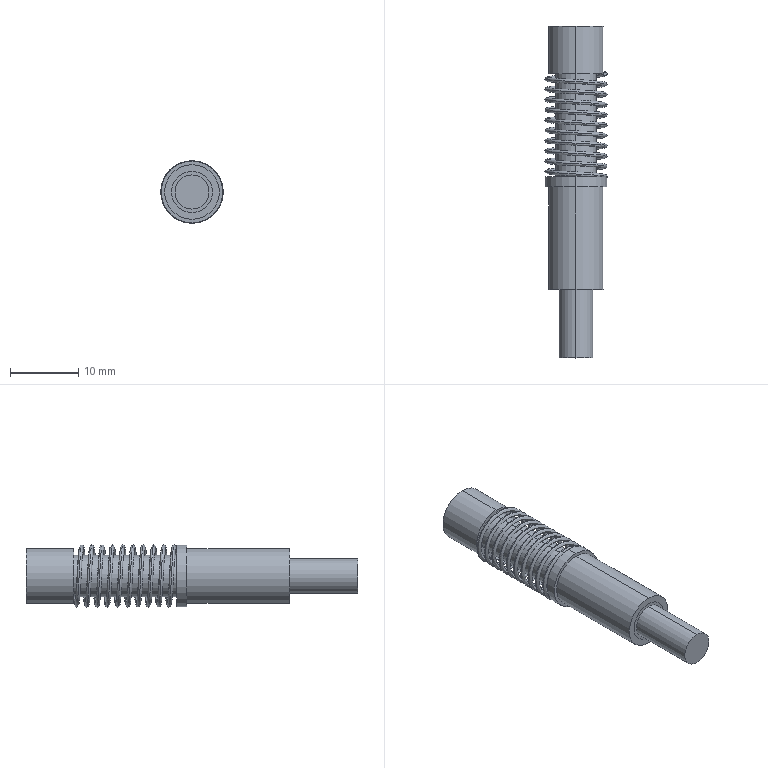Part | STEP file | 22CPMM160_Default | 4 solids | 24 faces | box 9.1 x 48.5 x 9.1 mm | volume 1897 mm3 | cylinder 12 | plane 10 | spline 2 | commonest cylinder face diameters 6 x4 8 x4 5 x2 9 x2